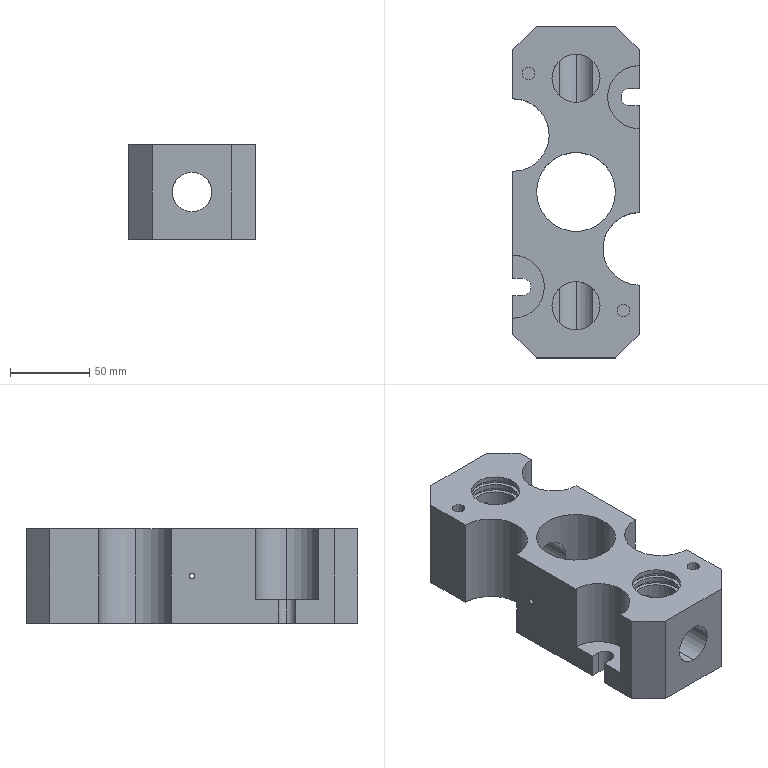Part | STEP file | Feed distributor part SGN-2-23 | 1 solid | 77 faces | box 80 x 210 x 60 mm | volume 591355 mm3 | cylinder 43 | plane 34 | commonest cylinder face diameters 30.5 x12 35 x8 3.3 x4 8 x4 25 x4 11 x3